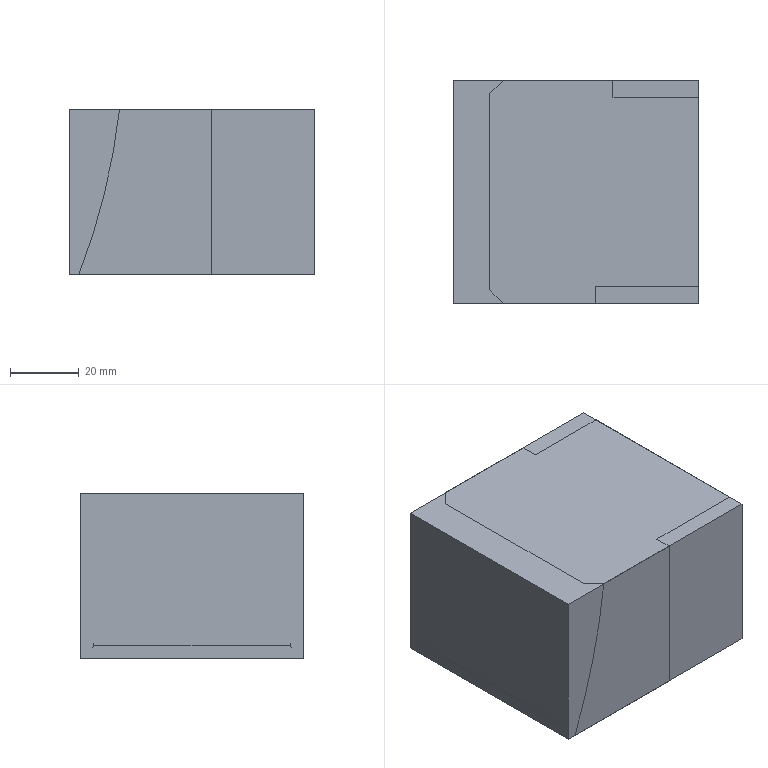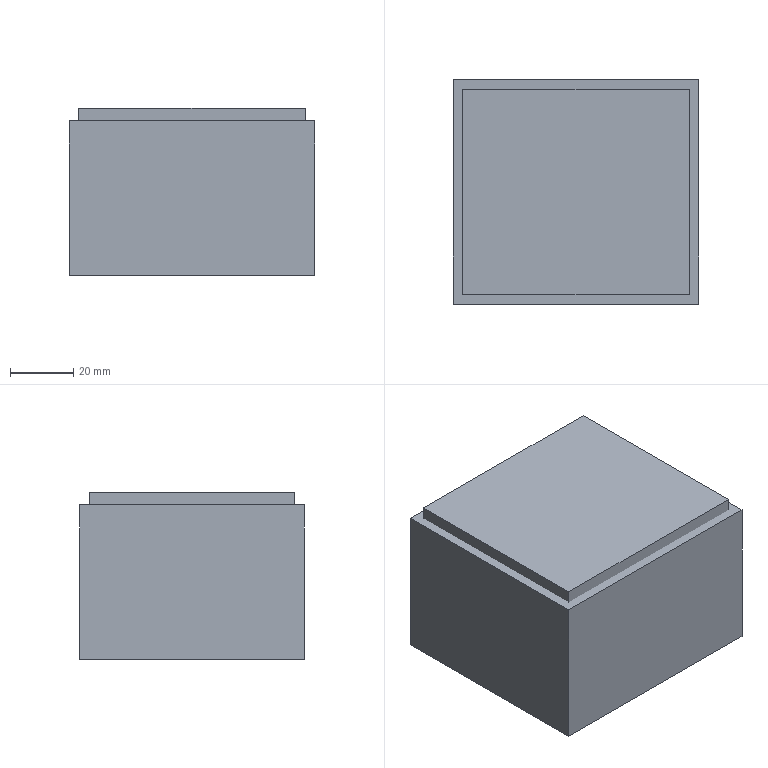CAM job | NX | 3+2 milling, drilling | part box 71.51 x 65 x 48 mm | stock box 77.51 x 71 x 53 mm
Tools:
number,name,description,diameter,corner_radius,flute_length,length,flutes
1,D63,Milling Tool-5 Parameters,63.0,0.0,50.0,75.0,2
10,D10,Milling Tool-5 Parameters,10.0,0.0,30.0,30.0,4
11,D10JING,Milling Tool-5 Parameters,10.0,0.0,50.0,75.0,2
7,D6A45,Milling Tool-5 Parameters,6.0,0.0,3.0,3.0,2
14,4.8ZT,Drilling Tool,4.8,0.0,35.0,50.0,2
15,5.0JD,Milling Tool-5 Parameters,5.0,0.0,30.0,30.0,4
17,7.0ZT,Drilling Tool,7.0,0.0,35.0,50.0,2
5,D6R0.5,Milling Tool-5 Parameters,6.0,0.5,50.0,75.0,2
Operations:
program,operation,operation_type,tool,method,geometry_group,spindle_rpm,surface_speed,feed_per_tooth,feed_cut,feed_plunge,cut_length_mm,path_length_mm,cut_time_min,machine_time_min
1,FLOOR_WALL,VolumeBased25DMillingOperation,D63,METHOD,A,6500.0,1286.0,0.0962,1250.0,100.0,338.817,392.817,0.2711,0.2765
1,ZLEVEL_PROFILE_COPY,ZLevelMilling,D10,METHOD,A,9500.0,298.0,0.0526,2000.0,100.0,14996.897,15101.897,7.498,7.509
1,ZLEVEL_PROFILE_COPY_COPY_COPY,ZLevelMilling,D10JING,METHOD,A,9500.0,298.0,0.0395,1500.0,1000.0,947.324,1098.022,0.6371,0.6522
1,ZLEVEL_PROFILE_1_COPY_1,ZLevelMilling,D6A45,METHOD,A,9500.0,179.0,0.0526,1000.0,100.0,284.141,344.141,0.2841,0.2901
2,FLOOR_WALL_COPY,VolumeBased25DMillingOperation,D63,METHOD,B,6500.0,1286.0,0.0962,1250.0,100.0,1604.086,2013.275,1.283,1.324
2,ZLEVEL_PROFILE_1_COPY_1_COPY,ZLevelMilling,D6A45,METHOD,B,9500.0,179.0,0.0526,1000.0,100.0,284.141,344.141,0.2841,0.2901
3,DRILLING_COPY_1,Operation,D6A45,METHOD,C,5000.0,94.0,0.025,250.0,0.0,24.0,228.228,0.096,0.1164
3,DRILLING_COPY_COPY_1,Operation,4.8ZT,METHOD,C,2000.0,15.0,0.03,120.0,0.0,32.884,168.881,0.274,0.2876
3,DRILLING_COPY_COPY_1_COPY,Operation,5.0JD,METHOD,C,1000.0,15.0,0.0125,50.0,0.0,30.0,163.112,0.6,0.6133
3,DRILLING_COPY_COPY_1_COPY_1,Operation,7.0ZT,METHOD,C,2000.0,43.0,0.05,200.0,0.0,68.412,310.217,0.3421,0.3662
3,ZLEVEL_PROFILE_COPY_COPY,ZLevelMilling,D10,METHOD,C,9500.0,298.0,0.0921,3500.0,1000.0,1907.71,2027.41,0.6018,0.6138
3,ZLEVEL_PROFILE_COPY_COPY_COPY_1,ZLevelMilling,D10,METHOD,C,9500.0,298.0,0.0921,3500.0,1000.0,1590.349,1700.049,0.5017,0.5126
3,ZLEVEL_PROFILE_COPY_COPY_COPY_COPY,ZLevelMilling,D10JING,METHOD,C,9500.0,298.0,0.0395,1500.0,1000.0,348.507,793.19,0.2417,0.2862
3,ZLEVEL_PROFILE_1_COPY_1_COPY_COPY,ZLevelMilling,D6A45,METHOD,C,9500.0,179.0,0.0526,1000.0,100.0,331.597,952.673,0.3316,0.3937
4,FIXED_CONTOUR_COPY,SurfaceContour,D6R0.5,METHOD,D,9500.0,179.0,0.1842,3500.0,500.0,49365.005,49431.005,14.111,14.118